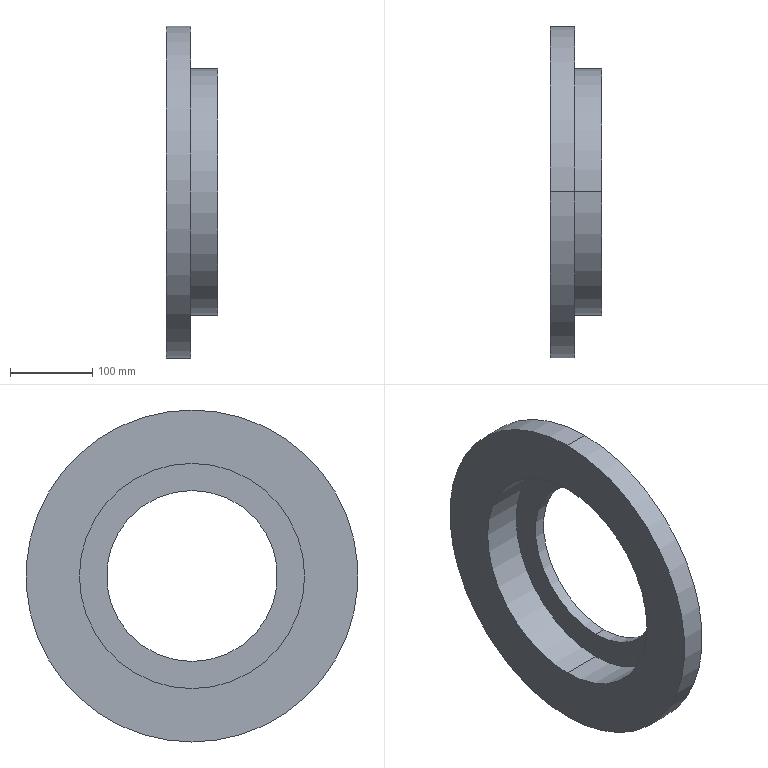Part | SolidWorks | features Revolution 1 | 1 solid | 21 faces | box 63 x 404 x 404 mm | volume 2394632 mm3 | cylinder 14 | plane 7 | commonest cylinder face diameters 208 x2 274 x2 300 x2 328 x2 352 x2 380 x2
STEP:
#1=CARTESIAN_POINT('',(63.,0.,-104.));
#2=VERTEX_POINT('',#1);
#3=CARTESIAN_POINT('',(63.,0.,104.));
#4=VERTEX_POINT('',#3);
#5=CARTESIAN_POINT('',(63.,0.,0.));
#6=DIRECTION('',(-1.,0.,0.));
#7=DIRECTION('',(0.,0.,1.));
#8=AXIS2_PLACEMENT_3D('',#5,#6,#7);
#9=CIRCLE('',#8,104.);
#10=EDGE_CURVE('',#2,#4,#9,.T.);
#11=ORIENTED_EDGE('',*,*,#10,.F.);
#12=CARTESIAN_POINT('',(49.,0.,-104.));
#13=VERTEX_POINT('',#12);
#14=CARTESIAN_POINT('',(0.,0.,-104.));
#15=DIRECTION('',(-1.,0.,0.));
#16=VECTOR('',#15,1000.);
#17=LINE('',#14,#16);
#18=EDGE_CURVE('',#2,#13,#17,.T.);
#19=ORIENTED_EDGE('',*,*,#18,.T.);
#20=CARTESIAN_POINT('',(49.,0.,104.));
#21=VERTEX_POINT('',#20);
#22=CARTESIAN_POINT('',(49.,0.,0.));
#23=DIRECTION('',(-1.,0.,0.));
#24=DIRECTION('',(0.,0.,1.));
#25=AXIS2_PLACEMENT_3D('',#22,#23,#24);
#26=CIRCLE('',#25,104.);
#27=EDGE_CURVE('',#13,#21,#26,.T.);
#28=ORIENTED_EDGE('',*,*,#27,.T.);
#29=CARTESIAN_POINT('',(0.,0.,104.));
#30=DIRECTION('',(-1.,0.,0.));
#31=VECTOR('',#30,1000.);
#32=LINE('',#29,#31);
#33=EDGE_CURVE('',#4,#21,#32,.T.);
#34=ORIENTED_EDGE('',*,*,#33,.F.);
#35=EDGE_LOOP('',(#11,#19,#28,#34));
#36=FACE_OUTER_BOUND('',#35,.T.);
#37=CARTESIAN_POINT('',(0.,0.,0.));
#38=DIRECTION('',(-1.,0.,0.));
#39=DIRECTION('',(0.,0.,1.));
#40=AXIS2_PLACEMENT_3D('',#37,#38,#39);
#41=CYLINDRICAL_SURFACE('',#40,104.);
#42=ADVANCED_FACE('',(#36),#41,.F.);
#43=CARTESIAN_POINT('',(63.,0.,150.));
#44=VERTEX_POINT('',#43);
#45=CARTESIAN_POINT('',(63.,0.,-150.));
#46=VERTEX_POINT('',#45);
#47=CARTESIAN_POINT('',(63.,0.,0.));
#48=DIRECTION('',(-1.,0.,0.));
#49=DIRECTION('',(0.,0.,1.));
#50=AXIS2_PLACEMENT_3D('',#47,#48,#49);
#51=CIRCLE('',#50,150.);
#52=EDGE_CURVE('',#44,#46,#51,.T.);
#53=ORIENTED_EDGE('',*,*,#52,.T.);
#54=CARTESIAN_POINT('',(16.,0.,-150.));
#55=VERTEX_POINT('',#54);
#56=CARTESIAN_POINT('',(0.,0.,-150.));
#57=DIRECTION('',(-1.,0.,0.));
#58=VECTOR('',#57,1000.);
#59=LINE('',#56,#58);
#60=EDGE_CURVE('',#46,#55,#59,.T.);
#61=ORIENTED_EDGE('',*,*,#60,.T.);
#62=CARTESIAN_POINT('',(16.,0.,150.));
#63=VERTEX_POINT('',#62);
#64=CARTESIAN_POINT('',(16.,0.,0.));
#65=DIRECTION('',(-1.,0.,0.));
#66=DIRECTION('',(0.,0.,1.));
#67=AXIS2_PLACEMENT_3D('',#64,#65,#66);
#68=CIRCLE('',#67,150.);
#69=EDGE_CURVE('',#63,#55,#68,.T.);
#70=ORIENTED_EDGE('',*,*,#69,.F.);
#71=CARTESIAN_POINT('',(0.,0.,150.));
#72=DIRECTION('',(-1.,0.,0.));
#73=VECTOR('',#72,1000.);
#74=LINE('',#71,#73);
#75=EDGE_CURVE('',#44,#63,#74,.T.);
#76=ORIENTED_EDGE('',*,*,#75,.F.);
#77=EDGE_LOOP('',(#53,#61,#70,#76));
#78=FACE_OUTER_BOUND('',#77,.T.);
#79=CARTESIAN_POINT('',(0.,0.,0.));
#80=DIRECTION('',(-1.,0.,0.));
#81=DIRECTION('',(0.,0.,1.));
#82=AXIS2_PLACEMENT_3D('',#79,#80,#81);
#83=CYLINDRICAL_SURFACE('',#82,150.);
#84=ADVANCED_FACE('',(#78),#83,.T.);
#85=CARTESIAN_POINT('',(30.,0.,-164.));
#86=VERTEX_POINT('',#85);
#87=CARTESIAN_POINT('',(30.,0.,164.));
#88=VERTEX_POINT('',#87);
#89=CARTESIAN_POINT('',(30.,0.,0.));
#90=DIRECTION('',(-1.,0.,0.));
#91=DIRECTION('',(0.,0.,1.));
#92=AXIS2_PLACEMENT_3D('',#89,#90,#91);
#93=CIRCLE('',#92,164.);
#94=EDGE_CURVE('',#86,#88,#93,.T.);
#95=ORIENTED_EDGE('',*,*,#94,.F.);
#96=CARTESIAN_POINT('',(16.,0.,-164.));
#97=VERTEX_POINT('',#96);
#98=CARTESIAN_POINT('',(0.,0.,-164.));
#99=DIRECTION('',(-1.,0.,0.));
#100=VECTOR('',#99,1000.);
#101=LINE('',#98,#100);
#102=EDGE_CURVE('',#86,#97,#101,.T.);
#103=ORIENTED_EDGE('',*,*,#102,.T.);
#104=CARTESIAN_POINT('',(16.,0.,164.));
#105=VERTEX_POINT('',#104);
#106=CARTESIAN_POINT('',(16.,0.,0.));
#107=DIRECTION('',(-1.,0.,0.));
#108=DIRECTION('',(0.,0.,1.));
#109=AXIS2_PLACEMENT_3D('',#106,#107,#108);
#110=CIRCLE('',#109,164.);
#111=EDGE_CURVE('',#97,#105,#110,.T.);
#112=ORIENTED_EDGE('',*,*,#111,.T.);
#113=CARTESIAN_POINT('',(0.,0.,164.));
#114=DIRECTION('',(-1.,0.,0.));
#115=VECTOR('',#114,1000.);
#116=LINE('',#113,#115);
#117=EDGE_CURVE('',#88,#105,#116,.T.);
#118=ORIENTED_EDGE('',*,*,#117,.F.);
#119=EDGE_LOOP('',(#95,#103,#112,#118));
#120=FACE_OUTER_BOUND('',#119,.T.);
#121=CARTESIAN_POINT('',(0.,0.,0.));
#122=DIRECTION('',(-1.,0.,0.));
#123=DIRECTION('',(0.,0.,1.));
#124=AXIS2_PLACEMENT_3D('',#121,#122,#123);
#125=CYLINDRICAL_SURFACE('',#124,164.);
#126=ADVANCED_FACE('',(#120),#125,.F.);
#127=CARTESIAN_POINT('',(30.,0.,176.));
#128=VERTEX_POINT('',#127);
#129=CARTESIAN_POINT('',(30.,0.,-176.));
#130=VERTEX_POINT('',#129);
#131=CARTESIAN_POINT('',(30.,0.,0.));
#132=DIRECTION('',(-1.,0.,0.));
#133=DIRECTION('',(0.,0.,1.));
#134=AXIS2_PLACEMENT_3D('',#131,#132,#133);
#135=CIRCLE('',#134,176.);
#136=EDGE_CURVE('',#128,#130,#135,.T.);
#137=ORIENTED_EDGE('',*,*,#136,.T.);
#138=CARTESIAN_POINT('',(16.,0.,-176.));
#139=VERTEX_POINT('',#138);
#140=CARTESIAN_POINT('',(0.,0.,-176.));
#141=DIRECTION('',(-1.,0.,0.));
#142=VECTOR('',#141,1000.);
#143=LINE('',#140,#142);
#144=EDGE_CURVE('',#130,#139,#143,.T.);
#145=ORIENTED_EDGE('',*,*,#144,.T.);
#146=CARTESIAN_POINT('',(16.,0.,176.));
#147=VERTEX_POINT('',#146);
#148=CARTESIAN_POINT('',(16.,0.,0.));
#149=DIRECTION('',(-1.,0.,0.));
#150=DIRECTION('',(0.,0.,1.));
#151=AXIS2_PLACEMENT_3D('',#148,#149,#150);
#152=CIRCLE('',#151,176.);
#153=EDGE_CURVE('',#147,#139,#152,.T.);
#154=ORIENTED_EDGE('',*,*,#153,.F.);
#155=CARTESIAN_POINT('',(0.,0.,176.));
#156=DIRECTION('',(-1.,0.,0.));
#157=VECTOR('',#156,1000.);
#158=LINE('',#155,#157);
#159=EDGE_CURVE('',#128,#147,#158,.T.);
#160=ORIENTED_EDGE('',*,*,#159,.F.);
#161=EDGE_LOOP('',(#137,#145,#154,#160));
#162=FACE_OUTER_BOUND('',#161,.T.);
#163=CARTESIAN_POINT('',(0.,0.,0.));
#164=DIRECTION('',(-1.,0.,0.));
#165=DIRECTION('',(0.,0.,1.));
#166=AXIS2_PLACEMENT_3D('',#163,#164,#165);
#167=CYLINDRICAL_SURFACE('',#166,176.);
#168=ADVANCED_FACE('',(#162),#167,.T.);
#169=CARTESIAN_POINT('',(30.,0.,-190.));
#170=VERTEX_POINT('',#169);
#171=CARTESIAN_POINT('',(30.,0.,190.));
#172=VERTEX_POINT('',#171);
#173=CARTESIAN_POINT('',(30.,0.,0.));
#174=DIRECTION('',(-1.,0.,0.));
#175=DIRECTION('',(0.,0.,1.));
#176=AXIS2_PLACEMENT_3D('',#173,#174,#175);
#177=CIRCLE('',#176,190.);
#178=EDGE_CURVE('',#170,#172,#177,.T.);
#179=ORIENTED_EDGE('',*,*,#178,.F.);
#180=CARTESIAN_POINT('',(16.,0.,-190.));
#181=VERTEX_POINT('',#180);
#182=CARTESIAN_POINT('',(0.,0.,-190.));
#183=DIRECTION('',(-1.,0.,0.));
#184=VECTOR('',#183,1000.);
#185=LINE('',#182,#184);
#186=EDGE_CURVE('',#170,#181,#185,.T.);
#187=ORIENTED_EDGE('',*,*,#186,.T.);
#188=CARTESIAN_POINT('',(16.,0.,190.));
#189=VERTEX_POINT('',#188);
#190=CARTESIAN_POINT('',(16.,0.,0.));
#191=DIRECTION('',(-1.,0.,0.));
#192=DIRECTION('',(0.,0.,1.));
#193=AXIS2_PLACEMENT_3D('',#190,#191,#192);
#194=CIRCLE('',#193,190.);
#195=EDGE_CURVE('',#181,#189,#194,.T.);
#196=ORIENTED_EDGE('',*,*,#195,.T.);
#197=CARTESIAN_POINT('',(0.,0.,190.));
#198=DIRECTION('',(-1.,0.,0.));
#199=VECTOR('',#198,1000.);
#200=LINE('',#197,#199);
#201=EDGE_CURVE('',#172,#189,#200,.T.);
#202=ORIENTED_EDGE('',*,*,#201,.F.);
#203=EDGE_LOOP('',(#179,#187,#196,#202));
#204=FACE_OUTER_BOUND('',#203,.T.);
#205=CARTESIAN_POINT('',(0.,0.,0.));
#206=DIRECTION('',(-1.,0.,0.));
#207=DIRECTION('',(0.,0.,1.));
#208=AXIS2_PLACEMENT_3D('',#205,#206,#207);
#209=CYLINDRICAL_SURFACE('',#208,190.);
#210=ADVANCED_FACE('',(#204),#209,.F.);
#211=CARTESIAN_POINT('',(30.,0.,202.));
#212=VERTEX_POINT('',#211);
#213=CARTESIAN_POINT('',(30.,0.,-202.));
#214=VERTEX_POINT('',#213);
#215=CARTESIAN_POINT('',(30.,0.,0.));
#216=DIRECTION('',(-1.,0.,0.));
#217=DIRECTION('',(0.,0.,1.));
#218=AXIS2_PLACEMENT_3D('',#215,#216,#217);
#219=CIRCLE('',#218,202.);
#220=EDGE_CURVE('',#212,#214,#219,.T.);
#221=ORIENTED_EDGE('',*,*,#220,.T.);
#222=CARTESIAN_POINT('',(0.,0.,-202.));
#223=VERTEX_POINT('',#222);
#224=CARTESIAN_POINT('',(0.,0.,-202.));
#225=DIRECTION('',(-1.,0.,0.));
#226=VECTOR('',#225,1000.);
#227=LINE('',#224,#226);
#228=EDGE_CURVE('',#214,#223,#227,.T.);
#229=ORIENTED_EDGE('',*,*,#228,.T.);
#230=CARTESIAN_POINT('',(0.,0.,202.));
#231=VERTEX_POINT('',#230);
#232=CARTESIAN_POINT('',(0.,0.,0.));
#233=DIRECTION('',(-1.,0.,0.));
#234=DIRECTION('',(0.,0.,1.));
#235=AXIS2_PLACEMENT_3D('',#232,#233,#234);
#236=CIRCLE('',#235,202.);
#237=EDGE_CURVE('',#231,#223,#236,.T.);
#238=ORIENTED_EDGE('',*,*,#237,.F.);
#239=CARTESIAN_POINT('',(0.,0.,202.));
#240=DIRECTION('',(-1.,0.,0.));
#241=VECTOR('',#240,1000.);
#242=LINE('',#239,#241);
#243=EDGE_CURVE('',#212,#231,#242,.T.);
#244=ORIENTED_EDGE('',*,*,#243,.F.);
#245=EDGE_LOOP('',(#221,#229,#238,#244));
#246=FACE_OUTER_BOUND('',#245,.T.);
#247=CARTESIAN_POINT('',(0.,0.,0.));
#248=DIRECTION('',(-1.,0.,0.));
#249=DIRECTION('',(0.,0.,1.));
#250=AXIS2_PLACEMENT_3D('',#247,#248,#249);
#251=CYLINDRICAL_SURFACE('',#250,202.);
#252=ADVANCED_FACE('',(#246),#251,.T.);
#253=CARTESIAN_POINT('',(49.,0.,-137.));
#254=VERTEX_POINT('',#253);
#255=CARTESIAN_POINT('',(49.,0.,137.));
#256=VERTEX_POINT('',#255);
#257=CARTESIAN_POINT('',(49.,0.,0.));
#258=DIRECTION('',(-1.,0.,0.));
#259=DIRECTION('',(0.,0.,1.));
#260=AXIS2_PLACEMENT_3D('',#257,#258,#259);
#261=CIRCLE('',#260,137.);
#262=EDGE_CURVE('',#254,#256,#261,.T.);
#263=ORIENTED_EDGE('',*,*,#262,.F.);
#264=CARTESIAN_POINT('',(0.,0.,-137.));
#265=VERTEX_POINT('',#264);
#266=CARTESIAN_POINT('',(0.,0.,-137.));
#267=DIRECTION('',(-1.,0.,0.));
#268=VECTOR('',#267,1000.);
#269=LINE('',#266,#268);
#270=EDGE_CURVE('',#254,#265,#269,.T.);
#271=ORIENTED_EDGE('',*,*,#270,.T.);
#272=CARTESIAN_POINT('',(0.,0.,137.));
#273=VERTEX_POINT('',#272);
#274=CARTESIAN_POINT('',(0.,0.,0.));
#275=DIRECTION('',(-1.,0.,0.));
#276=DIRECTION('',(0.,0.,1.));
#277=AXIS2_PLACEMENT_3D('',#274,#275,#276);
#278=CIRCLE('',#277,137.);
#279=EDGE_CURVE('',#265,#273,#278,.T.);
#280=ORIENTED_EDGE('',*,*,#279,.T.);
#281=CARTESIAN_POINT('',(0.,0.,137.));
#282=DIRECTION('',(-1.,0.,0.));
#283=VECTOR('',#282,1000.);
#284=LINE('',#281,#283);
#285=EDGE_CURVE('',#256,#273,#284,.T.);
#286=ORIENTED_EDGE('',*,*,#285,.F.);
#287=EDGE_LOOP('',(#263,#271,#280,#286));
#288=FACE_OUTER_BOUND('',#287,.T.);
#289=CARTESIAN_POINT('',(0.,0.,0.));
#290=DIRECTION('',(-1.,0.,0.));
#291=DIRECTION('',(0.,0.,1.));
#292=AXIS2_PLACEMENT_3D('',#289,#290,#291);
#293=CYLINDRICAL_SURFACE('',#292,137.);
#294=ADVANCED_FACE('',(#288),#293,.F.);
#295=ORIENTED_EDGE('',*,*,#270,.F.);
#296=CARTESIAN_POINT('',(49.,0.,0.));
#297=DIRECTION('',(-1.,0.,0.));
#298=DIRECTION('',(0.,0.,1.));
#299=AXIS2_PLACEMENT_3D('',#296,#297,#298);
#300=CIRCLE('',#299,137.);
#301=EDGE_CURVE('',#256,#254,#300,.T.);
#302=ORIENTED_EDGE('',*,*,#301,.F.);
#303=ORIENTED_EDGE('',*,*,#285,.T.);
#304=CARTESIAN_POINT('',(0.,0.,0.));
#305=DIRECTION('',(-1.,0.,0.));
#306=DIRECTION('',(0.,0.,1.));
#307=AXIS2_PLACEMENT_3D('',#304,#305,#306);
#308=CIRCLE('',#307,137.);
#309=EDGE_CURVE('',#273,#265,#308,.T.);
#310=ORIENTED_EDGE('',*,*,#309,.T.);
#311=EDGE_LOOP('',(#295,#302,#303,#310));
#312=FACE_OUTER_BOUND('',#311,.T.);
#313=CARTESIAN_POINT('',(0.,0.,0.));
#314=DIRECTION('',(-1.,0.,0.));
#315=DIRECTION('',(0.,0.,1.));
#316=AXIS2_PLACEMENT_3D('',#313,#314,#315);
#317=CYLINDRICAL_SURFACE('',#316,137.);
#318=ADVANCED_FACE('',(#312),#317,.F.);
#319=ORIENTED_EDGE('',*,*,#309,.F.);
#320=ORIENTED_EDGE('',*,*,#279,.F.);
#321=EDGE_LOOP('',(#319,#320));
#322=FACE_BOUND('',#321,.T.);
#323=ORIENTED_EDGE('',*,*,#237,.T.);
#324=CARTESIAN_POINT('',(0.,0.,0.));
#325=DIRECTION('',(-1.,0.,0.));
#326=DIRECTION('',(0.,0.,1.));
#327=AXIS2_PLACEMENT_3D('',#324,#325,#326);
#328=CIRCLE('',#327,202.);
#329=EDGE_CURVE('',#223,#231,#328,.T.);
#330=ORIENTED_EDGE('',*,*,#329,.T.);
#331=EDGE_LOOP('',(#323,#330));
#332=FACE_OUTER_BOUND('',#331,.T.);
#333=CARTESIAN_POINT('',(0.,137.,0.));
#334=DIRECTION('',(1.,0.,0.));
#335=DIRECTION('',(0.,0.,-1.));
#336=AXIS2_PLACEMENT_3D('',#333,#334,#335);
#337=PLANE('',#336);
#338=ADVANCED_FACE('',(#322,#332),#337,.F.);
#339=ORIENTED_EDGE('',*,*,#228,.F.);
#340=CARTESIAN_POINT('',(30.,0.,0.));
#341=DIRECTION('',(-1.,0.,0.));
#342=DIRECTION('',(0.,0.,1.));
#343=AXIS2_PLACEMENT_3D('',#340,#341,#342);
#344=CIRCLE('',#343,202.);
#345=EDGE_CURVE('',#214,#212,#344,.T.);
#346=ORIENTED_EDGE('',*,*,#345,.T.);
#347=ORIENTED_EDGE('',*,*,#243,.T.);
#348=ORIENTED_EDGE('',*,*,#329,.F.);
#349=EDGE_LOOP('',(#339,#346,#347,#348));
#350=FACE_OUTER_BOUND('',#349,.T.);
#351=CARTESIAN_POINT('',(0.,0.,0.));
#352=DIRECTION('',(-1.,0.,0.));
#353=DIRECTION('',(0.,0.,1.));
#354=AXIS2_PLACEMENT_3D('',#351,#352,#353);
#355=CYLINDRICAL_SURFACE('',#354,202.);
#356=ADVANCED_FACE('',(#350),#355,.T.);
#357=ORIENTED_EDGE('',*,*,#220,.F.);
#358=ORIENTED_EDGE('',*,*,#345,.F.);
#359=EDGE_LOOP('',(#357,#358));
#360=FACE_OUTER_BOUND('',#359,.T.);
#361=CARTESIAN_POINT('',(30.,0.,0.));
#362=DIRECTION('',(-1.,0.,0.));
#363=DIRECTION('',(0.,0.,1.));
#364=AXIS2_PLACEMENT_3D('',#361,#362,#363);
#365=CIRCLE('',#364,190.);
#366=EDGE_CURVE('',#172,#170,#365,.T.);
#367=ORIENTED_EDGE('',*,*,#366,.T.);
#368=ORIENTED_EDGE('',*,*,#178,.T.);
#369=EDGE_LOOP('',(#367,#368));
#370=FACE_BOUND('',#369,.T.);
#371=CARTESIAN_POINT('',(30.,202.,0.));
#372=DIRECTION('',(-1.,0.,0.));
#373=DIRECTION('',(0.,0.,1.));
#374=AXIS2_PLACEMENT_3D('',#371,#372,#373);
#375=PLANE('',#374);
#376=ADVANCED_FACE('',(#360,#370),#375,.F.);
#377=ORIENTED_EDGE('',*,*,#186,.F.);
#378=ORIENTED_EDGE('',*,*,#366,.F.);
#379=ORIENTED_EDGE('',*,*,#201,.T.);
#380=CARTESIAN_POINT('',(16.,0.,0.));
#381=DIRECTION('',(-1.,0.,0.));
#382=DIRECTION('',(0.,0.,1.));
#383=AXIS2_PLACEMENT_3D('',#380,#381,#382);
#384=CIRCLE('',#383,190.);
#385=EDGE_CURVE('',#189,#181,#384,.T.);
#386=ORIENTED_EDGE('',*,*,#385,.T.);
#387=EDGE_LOOP('',(#377,#378,#379,#386));
#388=FACE_OUTER_BOUND('',#387,.T.);
#389=CARTESIAN_POINT('',(0.,0.,0.));
#390=DIRECTION('',(-1.,0.,0.));
#391=DIRECTION('',(0.,0.,1.));
#392=AXIS2_PLACEMENT_3D('',#389,#390,#391);
#393=CYLINDRICAL_SURFACE('',#392,190.);
#394=ADVANCED_FACE('',(#388),#393,.F.);
#395=ORIENTED_EDGE('',*,*,#385,.F.);
#396=ORIENTED_EDGE('',*,*,#195,.F.);
#397=EDGE_LOOP('',(#395,#396));
#398=FACE_OUTER_BOUND('',#397,.T.);
#399=ORIENTED_EDGE('',*,*,#153,.T.);
#400=CARTESIAN_POINT('',(16.,0.,0.));
#401=DIRECTION('',(-1.,0.,0.));
#402=DIRECTION('',(0.,0.,1.));
#403=AXIS2_PLACEMENT_3D('',#400,#401,#402);
#404=CIRCLE('',#403,176.);
#405=EDGE_CURVE('',#139,#147,#404,.T.);
#406=ORIENTED_EDGE('',*,*,#405,.T.);
#407=EDGE_LOOP('',(#399,#406));
#408=FACE_BOUND('',#407,.T.);
#409=CARTESIAN_POINT('',(16.,190.,0.));
#410=DIRECTION('',(-1.,0.,0.));
#411=DIRECTION('',(0.,0.,1.));
#412=AXIS2_PLACEMENT_3D('',#409,#410,#411);
#413=PLANE('',#412);
#414=ADVANCED_FACE('',(#398,#408),#413,.F.);
#415=ORIENTED_EDGE('',*,*,#144,.F.);
#416=CARTESIAN_POINT('',(30.,0.,0.));
#417=DIRECTION('',(-1.,0.,0.));
#418=DIRECTION('',(0.,0.,1.));
#419=AXIS2_PLACEMENT_3D('',#416,#417,#418);
#420=CIRCLE('',#419,176.);
#421=EDGE_CURVE('',#130,#128,#420,.T.);
#422=ORIENTED_EDGE('',*,*,#421,.T.);
#423=ORIENTED_EDGE('',*,*,#159,.T.);
#424=ORIENTED_EDGE('',*,*,#405,.F.);
#425=EDGE_LOOP('',(#415,#422,#423,#424));
#426=FACE_OUTER_BOUND('',#425,.T.);
#427=CARTESIAN_POINT('',(0.,0.,0.));
#428=DIRECTION('',(-1.,0.,0.));
#429=DIRECTION('',(0.,0.,1.));
#430=AXIS2_PLACEMENT_3D('',#427,#428,#429);
#431=CYLINDRICAL_SURFACE('',#430,176.);
#432=ADVANCED_FACE('',(#426),#431,.T.);
#433=ORIENTED_EDGE('',*,*,#136,.F.);
#434=ORIENTED_EDGE('',*,*,#421,.F.);
#435=EDGE_LOOP('',(#433,#434));
#436=FACE_OUTER_BOUND('',#435,.T.);
#437=CARTESIAN_POINT('',(30.,0.,0.));
#438=DIRECTION('',(-1.,0.,0.));
#439=DIRECTION('',(0.,0.,1.));
#440=AXIS2_PLACEMENT_3D('',#437,#438,#439);
#441=CIRCLE('',#440,164.);
#442=EDGE_CURVE('',#88,#86,#441,.T.);
#443=ORIENTED_EDGE('',*,*,#442,.T.);
#444=ORIENTED_EDGE('',*,*,#94,.T.);
#445=EDGE_LOOP('',(#443,#444));
#446=FACE_BOUND('',#445,.T.);
#447=CARTESIAN_POINT('',(30.,176.,0.));
#448=DIRECTION('',(-1.,0.,0.));
#449=DIRECTION('',(0.,0.,1.));
#450=AXIS2_PLACEMENT_3D('',#447,#448,#449);
#451=PLANE('',#450);
#452=ADVANCED_FACE('',(#436,#446),#451,.F.);
#453=ORIENTED_EDGE('',*,*,#102,.F.);
#454=ORIENTED_EDGE('',*,*,#442,.F.);
#455=ORIENTED_EDGE('',*,*,#117,.T.);
#456=CARTESIAN_POINT('',(16.,0.,0.));
#457=DIRECTION('',(-1.,0.,0.));
#458=DIRECTION('',(0.,0.,1.));
#459=AXIS2_PLACEMENT_3D('',#456,#457,#458);
#460=CIRCLE('',#459,164.);
#461=EDGE_CURVE('',#105,#97,#460,.T.);
#462=ORIENTED_EDGE('',*,*,#461,.T.);
#463=EDGE_LOOP('',(#453,#454,#455,#462));
#464=FACE_OUTER_BOUND('',#463,.T.);
#465=CARTESIAN_POINT('',(0.,0.,0.));
#466=DIRECTION('',(-1.,0.,0.));
#467=DIRECTION('',(0.,0.,1.));
#468=AXIS2_PLACEMENT_3D('',#465,#466,#467);
#469=CYLINDRICAL_SURFACE('',#468,164.);
#470=ADVANCED_FACE('',(#464),#469,.F.);
#471=ORIENTED_EDGE('',*,*,#461,.F.);
#472=ORIENTED_EDGE('',*,*,#111,.F.);
#473=EDGE_LOOP('',(#471,#472));
#474=FACE_OUTER_BOUND('',#473,.T.);
#475=ORIENTED_EDGE('',*,*,#69,.T.);
#476=CARTESIAN_POINT('',(16.,0.,0.));
#477=DIRECTION('',(-1.,0.,0.));
#478=DIRECTION('',(0.,0.,1.));
#479=AXIS2_PLACEMENT_3D('',#476,#477,#478);
#480=CIRCLE('',#479,150.);
#481=EDGE_CURVE('',#55,#63,#480,.T.);
#482=ORIENTED_EDGE('',*,*,#481,.T.);
#483=EDGE_LOOP('',(#475,#482));
#484=FACE_BOUND('',#483,.T.);
#485=CARTESIAN_POINT('',(16.,164.,0.));
#486=DIRECTION('',(-1.,0.,0.));
#487=DIRECTION('',(0.,0.,1.));
#488=AXIS2_PLACEMENT_3D('',#485,#486,#487);
#489=PLANE('',#488);
#490=ADVANCED_FACE('',(#474,#484),#489,.F.);
#491=ORIENTED_EDGE('',*,*,#60,.F.);
#492=CARTESIAN_POINT('',(63.,0.,0.));
#493=DIRECTION('',(-1.,0.,0.));
#494=DIRECTION('',(0.,0.,1.));
#495=AXIS2_PLACEMENT_3D('',#492,#493,#494);
#496=CIRCLE('',#495,150.);
#497=EDGE_CURVE('',#46,#44,#496,.T.);
#498=ORIENTED_EDGE('',*,*,#497,.T.);
#499=ORIENTED_EDGE('',*,*,#75,.T.);
#500=ORIENTED_EDGE('',*,*,#481,.F.);
#501=EDGE_LOOP('',(#491,#498,#499,#500));
#502=FACE_OUTER_BOUND('',#501,.T.);
#503=CARTESIAN_POINT('',(0.,0.,0.));
#504=DIRECTION('',(-1.,0.,0.));
#505=DIRECTION('',(0.,0.,1.));
#506=AXIS2_PLACEMENT_3D('',#503,#504,#505);
#507=CYLINDRICAL_SURFACE('',#506,150.);
#508=ADVANCED_FACE('',(#502),#507,.T.);
#509=ORIENTED_EDGE('',*,*,#52,.F.);
#510=ORIENTED_EDGE('',*,*,#497,.F.);
#511=EDGE_LOOP('',(#509,#510));
#512=FACE_OUTER_BOUND('',#511,.T.);
#513=CARTESIAN_POINT('',(63.,0.,0.));
#514=DIRECTION('',(-1.,0.,0.));
#515=DIRECTION('',(0.,0.,1.));
#516=AXIS2_PLACEMENT_3D('',#513,#514,#515);
#517=CIRCLE('',#516,104.);
#518=EDGE_CURVE('',#4,#2,#517,.T.);
#519=ORIENTED_EDGE('',*,*,#518,.T.);
#520=ORIENTED_EDGE('',*,*,#10,.T.);
#521=EDGE_LOOP('',(#519,#520));
#522=FACE_BOUND('',#521,.T.);
#523=CARTESIAN_POINT('',(63.,150.,0.));
#524=DIRECTION('',(-1.,0.,0.));
#525=DIRECTION('',(0.,0.,1.));
#526=AXIS2_PLACEMENT_3D('',#523,#524,#525);
#527=PLANE('',#526);
#528=ADVANCED_FACE('',(#512,#522),#527,.F.);
#529=ORIENTED_EDGE('',*,*,#18,.F.);
#530=ORIENTED_EDGE('',*,*,#518,.F.);
#531=ORIENTED_EDGE('',*,*,#33,.T.);
#532=CARTESIAN_POINT('',(49.,0.,0.));
#533=DIRECTION('',(-1.,0.,0.));
#534=DIRECTION('',(0.,0.,1.));
#535=AXIS2_PLACEMENT_3D('',#532,#533,#534);
#536=CIRCLE('',#535,104.);
#537=EDGE_CURVE('',#21,#13,#536,.T.);
#538=ORIENTED_EDGE('',*,*,#537,.T.);
#539=EDGE_LOOP('',(#529,#530,#531,#538));
#540=FACE_OUTER_BOUND('',#539,.T.);
#541=CARTESIAN_POINT('',(0.,0.,0.));
#542=DIRECTION('',(-1.,0.,0.));
#543=DIRECTION('',(0.,0.,1.));
#544=AXIS2_PLACEMENT_3D('',#541,#542,#543);
#545=CYLINDRICAL_SURFACE('',#544,104.);
#546=ADVANCED_FACE('',(#540),#545,.F.);
#547=ORIENTED_EDGE('',*,*,#537,.F.);
#548=ORIENTED_EDGE('',*,*,#27,.F.);
#549=EDGE_LOOP('',(#547,#548));
#550=FACE_BOUND('',#549,.T.);
#551=ORIENTED_EDGE('',*,*,#301,.T.);
#552=ORIENTED_EDGE('',*,*,#262,.T.);
#553=EDGE_LOOP('',(#551,#552));
#554=FACE_OUTER_BOUND('',#553,.T.);
#555=CARTESIAN_POINT('',(49.,104.,0.));
#556=DIRECTION('',(1.,0.,0.));
#557=DIRECTION('',(0.,0.,-1.));
#558=AXIS2_PLACEMENT_3D('',#555,#556,#557);
#559=PLANE('',#558);
#560=ADVANCED_FACE('',(#550,#554),#559,.F.);
#561=CLOSED_SHELL('',(#42,#84,#126,#168,#210,#252,#294,#318,#338,#356,#376,#394,#414,#432,#452,#470,#490,#508,#528,#546,#560));
#562=MANIFOLD_SOLID_BREP('',#561);
#563=CARTESIAN_POINT('',(0.,0.,0.));
#564=DIRECTION('',(0.,0.,1.));
#565=DIRECTION('',(1.,0.,0.));
#566=AXIS2_PLACEMENT_3D('',#563,#564,#565);
#567=(LENGTH_UNIT()NAMED_UNIT(*)SI_UNIT(.MILLI.,.METRE.));
#568=UNCERTAINTY_MEASURE_WITH_UNIT(LENGTH_MEASURE(0.00001),#567,'','');
#569=(NAMED_UNIT(*)PLANE_ANGLE_UNIT()SI_UNIT($,.RADIAN.));
#570=(NAMED_UNIT(*)SI_UNIT($,.STERADIAN.)SOLID_ANGLE_UNIT());
#571=(GEOMETRIC_REPRESENTATION_CONTEXT(3)GLOBAL_UNCERTAINTY_ASSIGNED_CONTEXT((#568))GLOBAL_UNIT_ASSIGNED_CONTEXT((#567,#569,#570))REPRESENTATION_CONTEXT('',''));
#572=ADVANCED_BREP_SHAPE_REPRESENTATION('',(#562,#566),#571);